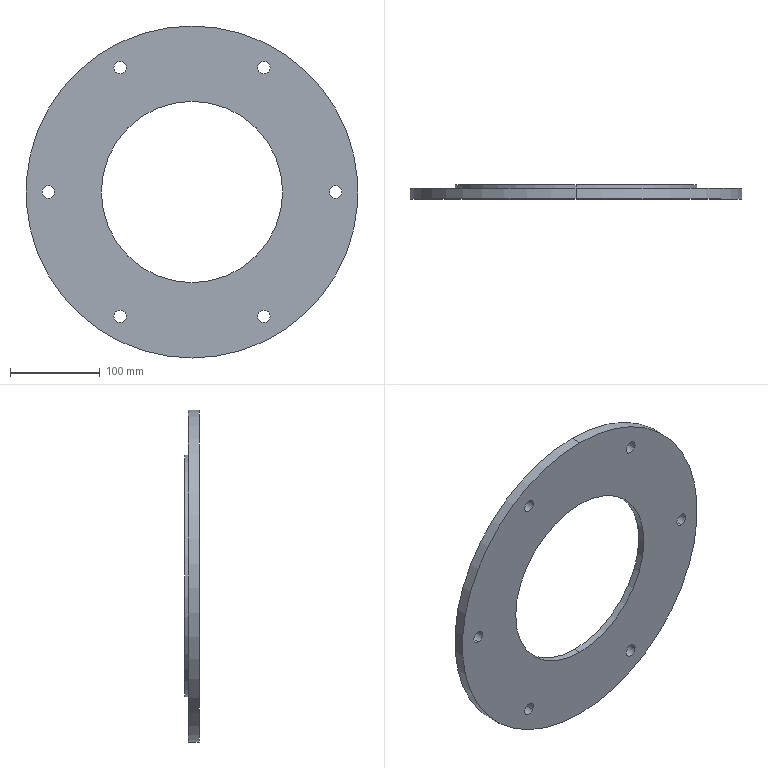Part | SolidWorks | features ICE 3, CirPattern 1, Extrusion 1 | 1 solid | 24 faces | box 370 x 16 x 370 mm | volume 827853 mm3 | cylinder 20 | plane 4 | commonest cylinder face diameters 14 x12 202 x2 259.5 x2 269.5 x2 370 x2
STEP:
#1=CARTESIAN_POINT('',(86.062,0.,135.064));
#2=VERTEX_POINT('',#1);
#3=CARTESIAN_POINT('',(73.938,0.,142.064));
#4=VERTEX_POINT('',#3);
#5=CARTESIAN_POINT('',(80.,0.,138.564));
#6=DIRECTION('',(0.,1.,0.));
#7=DIRECTION('',(-0.866,0.,0.5));
#8=AXIS2_PLACEMENT_3D('',#5,#6,#7);
#9=CIRCLE('',#8,7.);
#10=EDGE_CURVE('',#2,#4,#9,.T.);
#11=ORIENTED_EDGE('',*,*,#10,.F.);
#12=CARTESIAN_POINT('',(86.062,12.,135.064));
#13=VERTEX_POINT('',#12);
#14=CARTESIAN_POINT('',(86.062,0.,135.064));
#15=DIRECTION('',(0.,1.,0.));
#16=VECTOR('',#15,1000.);
#17=LINE('',#14,#16);
#18=EDGE_CURVE('',#2,#13,#17,.T.);
#19=ORIENTED_EDGE('',*,*,#18,.T.);
#20=CARTESIAN_POINT('',(73.938,12.,142.064));
#21=VERTEX_POINT('',#20);
#22=CARTESIAN_POINT('',(80.,12.,138.564));
#23=DIRECTION('',(0.,1.,0.));
#24=DIRECTION('',(-0.866,0.,0.5));
#25=AXIS2_PLACEMENT_3D('',#22,#23,#24);
#26=CIRCLE('',#25,7.);
#27=EDGE_CURVE('',#13,#21,#26,.T.);
#28=ORIENTED_EDGE('',*,*,#27,.T.);
#29=CARTESIAN_POINT('',(73.938,0.,142.064));
#30=DIRECTION('',(0.,1.,0.));
#31=VECTOR('',#30,1000.);
#32=LINE('',#29,#31);
#33=EDGE_CURVE('',#4,#21,#32,.T.);
#34=ORIENTED_EDGE('',*,*,#33,.F.);
#35=EDGE_LOOP('',(#11,#19,#28,#34));
#36=FACE_OUTER_BOUND('',#35,.T.);
#37=CARTESIAN_POINT('',(80.,0.,138.564));
#38=DIRECTION('',(0.,1.,0.));
#39=DIRECTION('',(-0.866,0.,0.5));
#40=AXIS2_PLACEMENT_3D('',#37,#38,#39);
#41=CYLINDRICAL_SURFACE('',#40,7.);
#42=ADVANCED_FACE('',(#36),#41,.F.);
#43=CARTESIAN_POINT('',(-73.938,0.,142.064));
#44=VERTEX_POINT('',#43);
#45=CARTESIAN_POINT('',(-86.062,0.,135.064));
#46=VERTEX_POINT('',#45);
#47=CARTESIAN_POINT('',(-80.,0.,138.564));
#48=DIRECTION('',(0.,1.,0.));
#49=DIRECTION('',(-0.866,0.,-0.5));
#50=AXIS2_PLACEMENT_3D('',#47,#48,#49);
#51=CIRCLE('',#50,7.);
#52=EDGE_CURVE('',#44,#46,#51,.T.);
#53=ORIENTED_EDGE('',*,*,#52,.F.);
#54=CARTESIAN_POINT('',(-73.938,12.,142.064));
#55=VERTEX_POINT('',#54);
#56=CARTESIAN_POINT('',(-73.938,0.,142.064));
#57=DIRECTION('',(0.,1.,0.));
#58=VECTOR('',#57,1000.);
#59=LINE('',#56,#58);
#60=EDGE_CURVE('',#44,#55,#59,.T.);
#61=ORIENTED_EDGE('',*,*,#60,.T.);
#62=CARTESIAN_POINT('',(-86.062,12.,135.064));
#63=VERTEX_POINT('',#62);
#64=CARTESIAN_POINT('',(-80.,12.,138.564));
#65=DIRECTION('',(0.,1.,0.));
#66=DIRECTION('',(-0.866,0.,-0.5));
#67=AXIS2_PLACEMENT_3D('',#64,#65,#66);
#68=CIRCLE('',#67,7.);
#69=EDGE_CURVE('',#55,#63,#68,.T.);
#70=ORIENTED_EDGE('',*,*,#69,.T.);
#71=CARTESIAN_POINT('',(-86.062,0.,135.064));
#72=DIRECTION('',(0.,1.,0.));
#73=VECTOR('',#72,1000.);
#74=LINE('',#71,#73);
#75=EDGE_CURVE('',#46,#63,#74,.T.);
#76=ORIENTED_EDGE('',*,*,#75,.F.);
#77=EDGE_LOOP('',(#53,#61,#70,#76));
#78=FACE_OUTER_BOUND('',#77,.T.);
#79=CARTESIAN_POINT('',(-80.,0.,138.564));
#80=DIRECTION('',(0.,1.,0.));
#81=DIRECTION('',(-0.866,0.,-0.5));
#82=AXIS2_PLACEMENT_3D('',#79,#80,#81);
#83=CYLINDRICAL_SURFACE('',#82,7.);
#84=ADVANCED_FACE('',(#78),#83,.F.);
#85=CARTESIAN_POINT('',(-160.,0.,7.));
#86=VERTEX_POINT('',#85);
#87=CARTESIAN_POINT('',(-160.,0.,-7.));
#88=VERTEX_POINT('',#87);
#89=CARTESIAN_POINT('',(-160.,0.,0.));
#90=DIRECTION('',(0.,1.,0.));
#91=DIRECTION('',(0.,0.,-1.));
#92=AXIS2_PLACEMENT_3D('',#89,#90,#91);
#93=CIRCLE('',#92,7.);
#94=EDGE_CURVE('',#86,#88,#93,.T.);
#95=ORIENTED_EDGE('',*,*,#94,.F.);
#96=CARTESIAN_POINT('',(-160.,12.,7.));
#97=VERTEX_POINT('',#96);
#98=CARTESIAN_POINT('',(-160.,0.,7.));
#99=DIRECTION('',(0.,1.,0.));
#100=VECTOR('',#99,1000.);
#101=LINE('',#98,#100);
#102=EDGE_CURVE('',#86,#97,#101,.T.);
#103=ORIENTED_EDGE('',*,*,#102,.T.);
#104=CARTESIAN_POINT('',(-160.,12.,-7.));
#105=VERTEX_POINT('',#104);
#106=CARTESIAN_POINT('',(-160.,12.,0.));
#107=DIRECTION('',(0.,1.,0.));
#108=DIRECTION('',(0.,0.,-1.));
#109=AXIS2_PLACEMENT_3D('',#106,#107,#108);
#110=CIRCLE('',#109,7.);
#111=EDGE_CURVE('',#97,#105,#110,.T.);
#112=ORIENTED_EDGE('',*,*,#111,.T.);
#113=CARTESIAN_POINT('',(-160.,0.,-7.));
#114=DIRECTION('',(0.,1.,0.));
#115=VECTOR('',#114,1000.);
#116=LINE('',#113,#115);
#117=EDGE_CURVE('',#88,#105,#116,.T.);
#118=ORIENTED_EDGE('',*,*,#117,.F.);
#119=EDGE_LOOP('',(#95,#103,#112,#118));
#120=FACE_OUTER_BOUND('',#119,.T.);
#121=CARTESIAN_POINT('',(-160.,0.,0.));
#122=DIRECTION('',(0.,1.,0.));
#123=DIRECTION('',(0.,0.,-1.));
#124=AXIS2_PLACEMENT_3D('',#121,#122,#123);
#125=CYLINDRICAL_SURFACE('',#124,7.);
#126=ADVANCED_FACE('',(#120),#125,.F.);
#127=CARTESIAN_POINT('',(-86.062,0.,-135.064));
#128=VERTEX_POINT('',#127);
#129=CARTESIAN_POINT('',(-73.938,0.,-142.064));
#130=VERTEX_POINT('',#129);
#131=CARTESIAN_POINT('',(-80.,0.,-138.564));
#132=DIRECTION('',(0.,1.,0.));
#133=DIRECTION('',(0.866,0.,-0.5));
#134=AXIS2_PLACEMENT_3D('',#131,#132,#133);
#135=CIRCLE('',#134,7.);
#136=EDGE_CURVE('',#128,#130,#135,.T.);
#137=ORIENTED_EDGE('',*,*,#136,.F.);
#138=CARTESIAN_POINT('',(-86.062,12.,-135.064));
#139=VERTEX_POINT('',#138);
#140=CARTESIAN_POINT('',(-86.062,0.,-135.064));
#141=DIRECTION('',(0.,1.,0.));
#142=VECTOR('',#141,1000.);
#143=LINE('',#140,#142);
#144=EDGE_CURVE('',#128,#139,#143,.T.);
#145=ORIENTED_EDGE('',*,*,#144,.T.);
#146=CARTESIAN_POINT('',(-73.938,12.,-142.064));
#147=VERTEX_POINT('',#146);
#148=CARTESIAN_POINT('',(-80.,12.,-138.564));
#149=DIRECTION('',(0.,1.,0.));
#150=DIRECTION('',(0.866,0.,-0.5));
#151=AXIS2_PLACEMENT_3D('',#148,#149,#150);
#152=CIRCLE('',#151,7.);
#153=EDGE_CURVE('',#139,#147,#152,.T.);
#154=ORIENTED_EDGE('',*,*,#153,.T.);
#155=CARTESIAN_POINT('',(-73.938,0.,-142.064));
#156=DIRECTION('',(0.,1.,0.));
#157=VECTOR('',#156,1000.);
#158=LINE('',#155,#157);
#159=EDGE_CURVE('',#130,#147,#158,.T.);
#160=ORIENTED_EDGE('',*,*,#159,.F.);
#161=EDGE_LOOP('',(#137,#145,#154,#160));
#162=FACE_OUTER_BOUND('',#161,.T.);
#163=CARTESIAN_POINT('',(-80.,0.,-138.564));
#164=DIRECTION('',(0.,1.,0.));
#165=DIRECTION('',(0.866,0.,-0.5));
#166=AXIS2_PLACEMENT_3D('',#163,#164,#165);
#167=CYLINDRICAL_SURFACE('',#166,7.);
#168=ADVANCED_FACE('',(#162),#167,.F.);
#169=CARTESIAN_POINT('',(73.938,0.,-142.064));
#170=VERTEX_POINT('',#169);
#171=CARTESIAN_POINT('',(86.062,0.,-135.064));
#172=VERTEX_POINT('',#171);
#173=CARTESIAN_POINT('',(80.,0.,-138.564));
#174=DIRECTION('',(0.,1.,0.));
#175=DIRECTION('',(0.866,0.,0.5));
#176=AXIS2_PLACEMENT_3D('',#173,#174,#175);
#177=CIRCLE('',#176,7.);
#178=EDGE_CURVE('',#170,#172,#177,.T.);
#179=ORIENTED_EDGE('',*,*,#178,.F.);
#180=CARTESIAN_POINT('',(73.938,12.,-142.064));
#181=VERTEX_POINT('',#180);
#182=CARTESIAN_POINT('',(73.938,0.,-142.064));
#183=DIRECTION('',(0.,1.,0.));
#184=VECTOR('',#183,1000.);
#185=LINE('',#182,#184);
#186=EDGE_CURVE('',#170,#181,#185,.T.);
#187=ORIENTED_EDGE('',*,*,#186,.T.);
#188=CARTESIAN_POINT('',(86.062,12.,-135.064));
#189=VERTEX_POINT('',#188);
#190=CARTESIAN_POINT('',(80.,12.,-138.564));
#191=DIRECTION('',(0.,1.,0.));
#192=DIRECTION('',(0.866,0.,0.5));
#193=AXIS2_PLACEMENT_3D('',#190,#191,#192);
#194=CIRCLE('',#193,7.);
#195=EDGE_CURVE('',#181,#189,#194,.T.);
#196=ORIENTED_EDGE('',*,*,#195,.T.);
#197=CARTESIAN_POINT('',(86.062,0.,-135.064));
#198=DIRECTION('',(0.,1.,0.));
#199=VECTOR('',#198,1000.);
#200=LINE('',#197,#199);
#201=EDGE_CURVE('',#172,#189,#200,.T.);
#202=ORIENTED_EDGE('',*,*,#201,.F.);
#203=EDGE_LOOP('',(#179,#187,#196,#202));
#204=FACE_OUTER_BOUND('',#203,.T.);
#205=CARTESIAN_POINT('',(80.,0.,-138.564));
#206=DIRECTION('',(0.,1.,0.));
#207=DIRECTION('',(0.866,0.,0.5));
#208=AXIS2_PLACEMENT_3D('',#205,#206,#207);
#209=CYLINDRICAL_SURFACE('',#208,7.);
#210=ADVANCED_FACE('',(#204),#209,.F.);
#211=CARTESIAN_POINT('',(160.,0.,-7.));
#212=VERTEX_POINT('',#211);
#213=CARTESIAN_POINT('',(160.,0.,7.));
#214=VERTEX_POINT('',#213);
#215=CARTESIAN_POINT('',(160.,0.,0.));
#216=DIRECTION('',(0.,1.,0.));
#217=DIRECTION('',(0.,0.,1.));
#218=AXIS2_PLACEMENT_3D('',#215,#216,#217);
#219=CIRCLE('',#218,7.);
#220=EDGE_CURVE('',#212,#214,#219,.T.);
#221=ORIENTED_EDGE('',*,*,#220,.F.);
#222=CARTESIAN_POINT('',(160.,12.,-7.));
#223=VERTEX_POINT('',#222);
#224=CARTESIAN_POINT('',(160.,0.,-7.));
#225=DIRECTION('',(0.,1.,0.));
#226=VECTOR('',#225,1000.);
#227=LINE('',#224,#226);
#228=EDGE_CURVE('',#212,#223,#227,.T.);
#229=ORIENTED_EDGE('',*,*,#228,.T.);
#230=CARTESIAN_POINT('',(160.,12.,7.));
#231=VERTEX_POINT('',#230);
#232=CARTESIAN_POINT('',(160.,12.,0.));
#233=DIRECTION('',(0.,1.,0.));
#234=DIRECTION('',(0.,0.,1.));
#235=AXIS2_PLACEMENT_3D('',#232,#233,#234);
#236=CIRCLE('',#235,7.);
#237=EDGE_CURVE('',#223,#231,#236,.T.);
#238=ORIENTED_EDGE('',*,*,#237,.T.);
#239=CARTESIAN_POINT('',(160.,0.,7.));
#240=DIRECTION('',(0.,1.,0.));
#241=VECTOR('',#240,1000.);
#242=LINE('',#239,#241);
#243=EDGE_CURVE('',#214,#231,#242,.T.);
#244=ORIENTED_EDGE('',*,*,#243,.F.);
#245=EDGE_LOOP('',(#221,#229,#238,#244));
#246=FACE_OUTER_BOUND('',#245,.T.);
#247=CARTESIAN_POINT('',(160.,0.,0.));
#248=DIRECTION('',(0.,1.,0.));
#249=DIRECTION('',(0.,0.,1.));
#250=AXIS2_PLACEMENT_3D('',#247,#248,#249);
#251=CYLINDRICAL_SURFACE('',#250,7.);
#252=ADVANCED_FACE('',(#246),#251,.F.);
#253=CARTESIAN_POINT('',(0.,16.,134.75));
#254=VERTEX_POINT('',#253);
#255=CARTESIAN_POINT('',(0.,16.,-134.75));
#256=VERTEX_POINT('',#255);
#257=CARTESIAN_POINT('',(0.,16.,0.));
#258=DIRECTION('',(0.,1.,0.));
#259=DIRECTION('',(0.,0.,1.));
#260=AXIS2_PLACEMENT_3D('',#257,#258,#259);
#261=CIRCLE('',#260,134.75);
#262=EDGE_CURVE('',#254,#256,#261,.T.);
#263=ORIENTED_EDGE('',*,*,#262,.F.);
#264=CARTESIAN_POINT('',(0.,12.,134.75));
#265=VERTEX_POINT('',#264);
#266=CARTESIAN_POINT('',(0.,16.,134.75));
#267=DIRECTION('',(0.,-1.,0.));
#268=VECTOR('',#267,1000.);
#269=LINE('',#266,#268);
#270=EDGE_CURVE('',#254,#265,#269,.T.);
#271=ORIENTED_EDGE('',*,*,#270,.T.);
#272=CARTESIAN_POINT('',(0.,12.,-134.75));
#273=VERTEX_POINT('',#272);
#274=CARTESIAN_POINT('',(0.,12.,0.));
#275=DIRECTION('',(0.,1.,0.));
#276=DIRECTION('',(0.,0.,1.));
#277=AXIS2_PLACEMENT_3D('',#274,#275,#276);
#278=CIRCLE('',#277,134.75);
#279=EDGE_CURVE('',#265,#273,#278,.T.);
#280=ORIENTED_EDGE('',*,*,#279,.T.);
#281=CARTESIAN_POINT('',(0.,16.,-134.75));
#282=DIRECTION('',(0.,-1.,0.));
#283=VECTOR('',#282,1000.);
#284=LINE('',#281,#283);
#285=EDGE_CURVE('',#256,#273,#284,.T.);
#286=ORIENTED_EDGE('',*,*,#285,.F.);
#287=EDGE_LOOP('',(#263,#271,#280,#286));
#288=FACE_OUTER_BOUND('',#287,.T.);
#289=CARTESIAN_POINT('',(0.,16.,0.));
#290=DIRECTION('',(0.,-1.,0.));
#291=DIRECTION('',(0.,0.,-1.));
#292=AXIS2_PLACEMENT_3D('',#289,#290,#291);
#293=CYLINDRICAL_SURFACE('',#292,134.75);
#294=ADVANCED_FACE('',(#288),#293,.T.);
#295=CARTESIAN_POINT('',(0.,8.,-129.75));
#296=VERTEX_POINT('',#295);
#297=CARTESIAN_POINT('',(0.,8.,129.75));
#298=VERTEX_POINT('',#297);
#299=CARTESIAN_POINT('',(0.,8.,0.));
#300=DIRECTION('',(0.,1.,0.));
#301=DIRECTION('',(0.,0.,1.));
#302=AXIS2_PLACEMENT_3D('',#299,#300,#301);
#303=CIRCLE('',#302,129.75);
#304=EDGE_CURVE('',#296,#298,#303,.T.);
#305=ORIENTED_EDGE('',*,*,#304,.F.);
#306=CARTESIAN_POINT('',(0.,16.,-129.75));
#307=VERTEX_POINT('',#306);
#308=CARTESIAN_POINT('',(0.,8.,-129.75));
#309=DIRECTION('',(0.,1.,0.));
#310=VECTOR('',#309,1000.);
#311=LINE('',#308,#310);
#312=EDGE_CURVE('',#296,#307,#311,.T.);
#313=ORIENTED_EDGE('',*,*,#312,.T.);
#314=CARTESIAN_POINT('',(0.,16.,129.75));
#315=VERTEX_POINT('',#314);
#316=CARTESIAN_POINT('',(0.,16.,0.));
#317=DIRECTION('',(0.,1.,0.));
#318=DIRECTION('',(0.,0.,1.));
#319=AXIS2_PLACEMENT_3D('',#316,#317,#318);
#320=CIRCLE('',#319,129.75);
#321=EDGE_CURVE('',#307,#315,#320,.T.);
#322=ORIENTED_EDGE('',*,*,#321,.T.);
#323=CARTESIAN_POINT('',(0.,8.,129.75));
#324=DIRECTION('',(0.,1.,0.));
#325=VECTOR('',#324,1000.);
#326=LINE('',#323,#325);
#327=EDGE_CURVE('',#298,#315,#326,.T.);
#328=ORIENTED_EDGE('',*,*,#327,.F.);
#329=EDGE_LOOP('',(#305,#313,#322,#328));
#330=FACE_OUTER_BOUND('',#329,.T.);
#331=CARTESIAN_POINT('',(0.,8.,0.));
#332=DIRECTION('',(0.,1.,0.));
#333=DIRECTION('',(0.,0.,1.));
#334=AXIS2_PLACEMENT_3D('',#331,#332,#333);
#335=CYLINDRICAL_SURFACE('',#334,129.75);
#336=ADVANCED_FACE('',(#330),#335,.F.);
#337=CARTESIAN_POINT('',(0.,12.,185.));
#338=VERTEX_POINT('',#337);
#339=CARTESIAN_POINT('',(0.,12.,-185.));
#340=VERTEX_POINT('',#339);
#341=CARTESIAN_POINT('',(0.,12.,0.));
#342=DIRECTION('',(0.,1.,0.));
#343=DIRECTION('',(0.,0.,1.));
#344=AXIS2_PLACEMENT_3D('',#341,#342,#343);
#345=CIRCLE('',#344,185.);
#346=EDGE_CURVE('',#338,#340,#345,.T.);
#347=ORIENTED_EDGE('',*,*,#346,.F.);
#348=CARTESIAN_POINT('',(0.,0.,185.));
#349=VERTEX_POINT('',#348);
#350=CARTESIAN_POINT('',(0.,12.,185.));
#351=DIRECTION('',(0.,-1.,0.));
#352=VECTOR('',#351,1000.);
#353=LINE('',#350,#352);
#354=EDGE_CURVE('',#338,#349,#353,.T.);
#355=ORIENTED_EDGE('',*,*,#354,.T.);
#356=CARTESIAN_POINT('',(0.,0.,-185.));
#357=VERTEX_POINT('',#356);
#358=CARTESIAN_POINT('',(0.,0.,0.));
#359=DIRECTION('',(0.,1.,0.));
#360=DIRECTION('',(0.,0.,1.));
#361=AXIS2_PLACEMENT_3D('',#358,#359,#360);
#362=CIRCLE('',#361,185.);
#363=EDGE_CURVE('',#349,#357,#362,.T.);
#364=ORIENTED_EDGE('',*,*,#363,.T.);
#365=CARTESIAN_POINT('',(0.,12.,-185.));
#366=DIRECTION('',(0.,-1.,0.));
#367=VECTOR('',#366,1000.);
#368=LINE('',#365,#367);
#369=EDGE_CURVE('',#340,#357,#368,.T.);
#370=ORIENTED_EDGE('',*,*,#369,.F.);
#371=EDGE_LOOP('',(#347,#355,#364,#370));
#372=FACE_OUTER_BOUND('',#371,.T.);
#373=CARTESIAN_POINT('',(0.,12.,0.));
#374=DIRECTION('',(0.,-1.,0.));
#375=DIRECTION('',(0.,0.,-1.));
#376=AXIS2_PLACEMENT_3D('',#373,#374,#375);
#377=CYLINDRICAL_SURFACE('',#376,185.);
#378=ADVANCED_FACE('',(#372),#377,.T.);
#379=CARTESIAN_POINT('',(0.,8.,-101.));
#380=VERTEX_POINT('',#379);
#381=CARTESIAN_POINT('',(0.,8.,101.));
#382=VERTEX_POINT('',#381);
#383=CARTESIAN_POINT('',(0.,8.,0.));
#384=DIRECTION('',(0.,1.,0.));
#385=DIRECTION('',(0.,0.,1.));
#386=AXIS2_PLACEMENT_3D('',#383,#384,#385);
#387=CIRCLE('',#386,101.);
#388=EDGE_CURVE('',#380,#382,#387,.T.);
#389=ORIENTED_EDGE('',*,*,#388,.T.);
#390=CARTESIAN_POINT('',(0.,0.,101.));
#391=VERTEX_POINT('',#390);
#392=CARTESIAN_POINT('',(0.,12.,101.));
#393=DIRECTION('',(0.,-1.,0.));
#394=VECTOR('',#393,1000.);
#395=LINE('',#392,#394);
#396=EDGE_CURVE('',#382,#391,#395,.T.);
#397=ORIENTED_EDGE('',*,*,#396,.T.);
#398=CARTESIAN_POINT('',(0.,0.,-101.));
#399=VERTEX_POINT('',#398);
#400=CARTESIAN_POINT('',(0.,0.,0.));
#401=DIRECTION('',(0.,1.,0.));
#402=DIRECTION('',(0.,0.,1.));
#403=AXIS2_PLACEMENT_3D('',#400,#401,#402);
#404=CIRCLE('',#403,101.);
#405=EDGE_CURVE('',#399,#391,#404,.T.);
#406=ORIENTED_EDGE('',*,*,#405,.F.);
#407=CARTESIAN_POINT('',(0.,12.,-101.));
#408=DIRECTION('',(0.,-1.,0.));
#409=VECTOR('',#408,1000.);
#410=LINE('',#407,#409);
#411=EDGE_CURVE('',#380,#399,#410,.T.);
#412=ORIENTED_EDGE('',*,*,#411,.F.);
#413=EDGE_LOOP('',(#389,#397,#406,#412));
#414=FACE_OUTER_BOUND('',#413,.T.);
#415=CARTESIAN_POINT('',(0.,12.,0.));
#416=DIRECTION('',(0.,-1.,0.));
#417=DIRECTION('',(0.,0.,-1.));
#418=AXIS2_PLACEMENT_3D('',#415,#416,#417);
#419=CYLINDRICAL_SURFACE('',#418,101.);
#420=ADVANCED_FACE('',(#414),#419,.F.);
#421=CARTESIAN_POINT('',(80.,12.,138.564));
#422=DIRECTION('',(0.,1.,0.));
#423=DIRECTION('',(-0.866,0.,0.5));
#424=AXIS2_PLACEMENT_3D('',#421,#422,#423);
#425=CIRCLE('',#424,7.);
#426=EDGE_CURVE('',#21,#13,#425,.T.);
#427=ORIENTED_EDGE('',*,*,#426,.F.);
#428=ORIENTED_EDGE('',*,*,#27,.F.);
#429=EDGE_LOOP('',(#427,#428));
#430=FACE_BOUND('',#429,.T.);
#431=CARTESIAN_POINT('',(-80.,12.,138.564));
#432=DIRECTION('',(0.,1.,0.));
#433=DIRECTION('',(-0.866,0.,-0.5));
#434=AXIS2_PLACEMENT_3D('',#431,#432,#433);
#435=CIRCLE('',#434,7.);
#436=EDGE_CURVE('',#63,#55,#435,.T.);
#437=ORIENTED_EDGE('',*,*,#436,.F.);
#438=ORIENTED_EDGE('',*,*,#69,.F.);
#439=EDGE_LOOP('',(#437,#438));
#440=FACE_BOUND('',#439,.T.);
#441=CARTESIAN_POINT('',(-160.,12.,0.));
#442=DIRECTION('',(0.,1.,0.));
#443=DIRECTION('',(0.,0.,-1.));
#444=AXIS2_PLACEMENT_3D('',#441,#442,#443);
#445=CIRCLE('',#444,7.);
#446=EDGE_CURVE('',#105,#97,#445,.T.);
#447=ORIENTED_EDGE('',*,*,#446,.F.);
#448=ORIENTED_EDGE('',*,*,#111,.F.);
#449=EDGE_LOOP('',(#447,#448));
#450=FACE_BOUND('',#449,.T.);
#451=CARTESIAN_POINT('',(-80.,12.,-138.564));
#452=DIRECTION('',(0.,1.,0.));
#453=DIRECTION('',(0.866,0.,-0.5));
#454=AXIS2_PLACEMENT_3D('',#451,#452,#453);
#455=CIRCLE('',#454,7.);
#456=EDGE_CURVE('',#147,#139,#455,.T.);
#457=ORIENTED_EDGE('',*,*,#456,.F.);
#458=ORIENTED_EDGE('',*,*,#153,.F.);
#459=EDGE_LOOP('',(#457,#458));
#460=FACE_BOUND('',#459,.T.);
#461=CARTESIAN_POINT('',(80.,12.,-138.564));
#462=DIRECTION('',(0.,1.,0.));
#463=DIRECTION('',(0.866,0.,0.5));
#464=AXIS2_PLACEMENT_3D('',#461,#462,#463);
#465=CIRCLE('',#464,7.);
#466=EDGE_CURVE('',#189,#181,#465,.T.);
#467=ORIENTED_EDGE('',*,*,#466,.F.);
#468=ORIENTED_EDGE('',*,*,#195,.F.);
#469=EDGE_LOOP('',(#467,#468));
#470=FACE_BOUND('',#469,.T.);
#471=CARTESIAN_POINT('',(160.,12.,0.));
#472=DIRECTION('',(0.,1.,0.));
#473=DIRECTION('',(0.,0.,1.));
#474=AXIS2_PLACEMENT_3D('',#471,#472,#473);
#475=CIRCLE('',#474,7.);
#476=EDGE_CURVE('',#231,#223,#475,.T.);
#477=ORIENTED_EDGE('',*,*,#476,.F.);
#478=ORIENTED_EDGE('',*,*,#237,.F.);
#479=EDGE_LOOP('',(#477,#478));
#480=FACE_BOUND('',#479,.T.);
#481=CARTESIAN_POINT('',(0.,12.,0.));
#482=DIRECTION('',(0.,1.,0.));
#483=DIRECTION('',(0.,0.,1.));
#484=AXIS2_PLACEMENT_3D('',#481,#482,#483);
#485=CIRCLE('',#484,185.);
#486=EDGE_CURVE('',#340,#338,#485,.T.);
#487=ORIENTED_EDGE('',*,*,#486,.T.);
#488=ORIENTED_EDGE('',*,*,#346,.T.);
#489=EDGE_LOOP('',(#487,#488));
#490=FACE_OUTER_BOUND('',#489,.T.);
#491=CARTESIAN_POINT('',(0.,12.,0.));
#492=DIRECTION('',(0.,1.,0.));
#493=DIRECTION('',(0.,0.,1.));
#494=AXIS2_PLACEMENT_3D('',#491,#492,#493);
#495=CIRCLE('',#494,134.75);
#496=EDGE_CURVE('',#273,#265,#495,.T.);
#497=ORIENTED_EDGE('',*,*,#496,.F.);
#498=ORIENTED_EDGE('',*,*,#279,.F.);
#499=EDGE_LOOP('',(#497,#498));
#500=FACE_BOUND('',#499,.T.);
#501=CARTESIAN_POINT('',(0.,12.,0.));
#502=DIRECTION('',(0.,1.,0.));
#503=DIRECTION('',(0.,0.,1.));
#504=AXIS2_PLACEMENT_3D('',#501,#502,#503);
#505=PLANE('',#504);
#506=ADVANCED_FACE('',(#430,#440,#450,#460,#470,#480,#490,#500),#505,.T.);
#507=ORIENTED_EDGE('',*,*,#396,.F.);
#508=CARTESIAN_POINT('',(0.,8.,0.));
#509=DIRECTION('',(0.,1.,0.));
#510=DIRECTION('',(0.,0.,1.));
#511=AXIS2_PLACEMENT_3D('',#508,#509,#510);
#512=CIRCLE('',#511,101.);
#513=EDGE_CURVE('',#382,#380,#512,.T.);
#514=ORIENTED_EDGE('',*,*,#513,.T.);
#515=ORIENTED_EDGE('',*,*,#411,.T.);
#516=CARTESIAN_POINT('',(0.,0.,0.));
#517=DIRECTION('',(0.,1.,0.));
#518=DIRECTION('',(0.,0.,1.));
#519=AXIS2_PLACEMENT_3D('',#516,#517,#518);
#520=CIRCLE('',#519,101.);
#521=EDGE_CURVE('',#391,#399,#520,.T.);
#522=ORIENTED_EDGE('',*,*,#521,.F.);
#523=EDGE_LOOP('',(#507,#514,#515,#522));
#524=FACE_OUTER_BOUND('',#523,.T.);
#525=CARTESIAN_POINT('',(0.,12.,0.));
#526=DIRECTION('',(0.,-1.,0.));
#527=DIRECTION('',(0.,0.,-1.));
#528=AXIS2_PLACEMENT_3D('',#525,#526,#527);
#529=CYLINDRICAL_SURFACE('',#528,101.);
#530=ADVANCED_FACE('',(#524),#529,.F.);
#531=CARTESIAN_POINT('',(80.,0.,138.564));
#532=DIRECTION('',(0.,1.,0.));
#533=DIRECTION('',(-0.866,0.,0.5));
#534=AXIS2_PLACEMENT_3D('',#531,#532,#533);
#535=CIRCLE('',#534,7.);
#536=EDGE_CURVE('',#4,#2,#535,.T.);
#537=ORIENTED_EDGE('',*,*,#536,.T.);
#538=ORIENTED_EDGE('',*,*,#10,.T.);
#539=EDGE_LOOP('',(#537,#538));
#540=FACE_BOUND('',#539,.T.);
#541=CARTESIAN_POINT('',(-80.,0.,138.564));
#542=DIRECTION('',(0.,1.,0.));
#543=DIRECTION('',(-0.866,0.,-0.5));
#544=AXIS2_PLACEMENT_3D('',#541,#542,#543);
#545=CIRCLE('',#544,7.);
#546=EDGE_CURVE('',#46,#44,#545,.T.);
#547=ORIENTED_EDGE('',*,*,#546,.T.);
#548=ORIENTED_EDGE('',*,*,#52,.T.);
#549=EDGE_LOOP('',(#547,#548));
#550=FACE_BOUND('',#549,.T.);
#551=CARTESIAN_POINT('',(-160.,0.,0.));
#552=DIRECTION('',(0.,1.,0.));
#553=DIRECTION('',(0.,0.,-1.));
#554=AXIS2_PLACEMENT_3D('',#551,#552,#553);
#555=CIRCLE('',#554,7.);
#556=EDGE_CURVE('',#88,#86,#555,.T.);
#557=ORIENTED_EDGE('',*,*,#556,.T.);
#558=ORIENTED_EDGE('',*,*,#94,.T.);
#559=EDGE_LOOP('',(#557,#558));
#560=FACE_BOUND('',#559,.T.);
#561=CARTESIAN_POINT('',(-80.,0.,-138.564));
#562=DIRECTION('',(0.,1.,0.));
#563=DIRECTION('',(0.866,0.,-0.5));
#564=AXIS2_PLACEMENT_3D('',#561,#562,#563);
#565=CIRCLE('',#564,7.);
#566=EDGE_CURVE('',#130,#128,#565,.T.);
#567=ORIENTED_EDGE('',*,*,#566,.T.);
#568=ORIENTED_EDGE('',*,*,#136,.T.);
#569=EDGE_LOOP('',(#567,#568));
#570=FACE_BOUND('',#569,.T.);
#571=CARTESIAN_POINT('',(80.,0.,-138.564));
#572=DIRECTION('',(0.,1.,0.));
#573=DIRECTION('',(0.866,0.,0.5));
#574=AXIS2_PLACEMENT_3D('',#571,#572,#573);
#575=CIRCLE('',#574,7.);
#576=EDGE_CURVE('',#172,#170,#575,.T.);
#577=ORIENTED_EDGE('',*,*,#576,.T.);
#578=ORIENTED_EDGE('',*,*,#178,.T.);
#579=EDGE_LOOP('',(#577,#578));
#580=FACE_BOUND('',#579,.T.);
#581=CARTESIAN_POINT('',(160.,0.,0.));
#582=DIRECTION('',(0.,1.,0.));
#583=DIRECTION('',(0.,0.,1.));
#584=AXIS2_PLACEMENT_3D('',#581,#582,#583);
#585=CIRCLE('',#584,7.);
#586=EDGE_CURVE('',#214,#212,#585,.T.);
#587=ORIENTED_EDGE('',*,*,#586,.T.);
#588=ORIENTED_EDGE('',*,*,#220,.T.);
#589=EDGE_LOOP('',(#587,#588));
#590=FACE_BOUND('',#589,.T.);
#591=CARTESIAN_POINT('',(0.,0.,0.));
#592=DIRECTION('',(0.,1.,0.));
#593=DIRECTION('',(0.,0.,1.));
#594=AXIS2_PLACEMENT_3D('',#591,#592,#593);
#595=CIRCLE('',#594,185.);
#596=EDGE_CURVE('',#357,#349,#595,.T.);
#597=ORIENTED_EDGE('',*,*,#596,.F.);
#598=ORIENTED_EDGE('',*,*,#363,.F.);
#599=EDGE_LOOP('',(#597,#598));
#600=FACE_OUTER_BOUND('',#599,.T.);
#601=ORIENTED_EDGE('',*,*,#405,.T.);
#602=ORIENTED_EDGE('',*,*,#521,.T.);
#603=EDGE_LOOP('',(#601,#602));
#604=FACE_BOUND('',#603,.T.);
#605=CARTESIAN_POINT('',(0.,0.,0.));
#606=DIRECTION('',(0.,1.,0.));
#607=DIRECTION('',(0.,0.,1.));
#608=AXIS2_PLACEMENT_3D('',#605,#606,#607);
#609=PLANE('',#608);
#610=ADVANCED_FACE('',(#540,#550,#560,#570,#580,#590,#600,#604),#609,.F.);
#611=ORIENTED_EDGE('',*,*,#354,.F.);
#612=ORIENTED_EDGE('',*,*,#486,.F.);
#613=ORIENTED_EDGE('',*,*,#369,.T.);
#614=ORIENTED_EDGE('',*,*,#596,.T.);
#615=EDGE_LOOP('',(#611,#612,#613,#614));
#616=FACE_OUTER_BOUND('',#615,.T.);
#617=CARTESIAN_POINT('',(0.,12.,0.));
#618=DIRECTION('',(0.,-1.,0.));
#619=DIRECTION('',(0.,0.,-1.));
#620=AXIS2_PLACEMENT_3D('',#617,#618,#619);
#621=CYLINDRICAL_SURFACE('',#620,185.);
#622=ADVANCED_FACE('',(#616),#621,.T.);
#623=ORIENTED_EDGE('',*,*,#312,.F.);
#624=CARTESIAN_POINT('',(0.,8.,0.));
#625=DIRECTION('',(0.,1.,0.));
#626=DIRECTION('',(0.,0.,1.));
#627=AXIS2_PLACEMENT_3D('',#624,#625,#626);
#628=CIRCLE('',#627,129.75);
#629=EDGE_CURVE('',#298,#296,#628,.T.);
#630=ORIENTED_EDGE('',*,*,#629,.F.);
#631=ORIENTED_EDGE('',*,*,#327,.T.);
#632=CARTESIAN_POINT('',(0.,16.,0.));
#633=DIRECTION('',(0.,1.,0.));
#634=DIRECTION('',(0.,0.,1.));
#635=AXIS2_PLACEMENT_3D('',#632,#633,#634);
#636=CIRCLE('',#635,129.75);
#637=EDGE_CURVE('',#315,#307,#636,.T.);
#638=ORIENTED_EDGE('',*,*,#637,.T.);
#639=EDGE_LOOP('',(#623,#630,#631,#638));
#640=FACE_OUTER_BOUND('',#639,.T.);
#641=CARTESIAN_POINT('',(0.,8.,0.));
#642=DIRECTION('',(0.,1.,0.));
#643=DIRECTION('',(0.,0.,1.));
#644=AXIS2_PLACEMENT_3D('',#641,#642,#643);
#645=CYLINDRICAL_SURFACE('',#644,129.75);
#646=ADVANCED_FACE('',(#640),#645,.F.);
#647=ORIENTED_EDGE('',*,*,#388,.F.);
#648=ORIENTED_EDGE('',*,*,#513,.F.);
#649=EDGE_LOOP('',(#647,#648));
#650=FACE_BOUND('',#649,.T.);
#651=ORIENTED_EDGE('',*,*,#629,.T.);
#652=ORIENTED_EDGE('',*,*,#304,.T.);
#653=EDGE_LOOP('',(#651,#652));
#654=FACE_OUTER_BOUND('',#653,.T.);
#655=CARTESIAN_POINT('',(0.,8.,0.));
#656=DIRECTION('',(0.,1.,0.));
#657=DIRECTION('',(0.,0.,1.));
#658=AXIS2_PLACEMENT_3D('',#655,#656,#657);
#659=PLANE('',#658);
#660=ADVANCED_FACE('',(#650,#654),#659,.T.);
#661=CARTESIAN_POINT('',(0.,16.,0.));
#662=DIRECTION('',(0.,1.,0.));
#663=DIRECTION('',(0.,0.,1.));
#664=AXIS2_PLACEMENT_3D('',#661,#662,#663);
#665=CIRCLE('',#664,134.75);
#666=EDGE_CURVE('',#256,#254,#665,.T.);
#667=ORIENTED_EDGE('',*,*,#666,.T.);
#668=ORIENTED_EDGE('',*,*,#262,.T.);
#669=EDGE_LOOP('',(#667,#668));
#670=FACE_OUTER_BOUND('',#669,.T.);
#671=ORIENTED_EDGE('',*,*,#637,.F.);
#672=ORIENTED_EDGE('',*,*,#321,.F.);
#673=EDGE_LOOP('',(#671,#672));
#674=FACE_BOUND('',#673,.T.);
#675=CARTESIAN_POINT('',(0.,16.,0.));
#676=DIRECTION('',(0.,1.,0.));
#677=DIRECTION('',(0.,0.,1.));
#678=AXIS2_PLACEMENT_3D('',#675,#676,#677);
#679=PLANE('',#678);
#680=ADVANCED_FACE('',(#670,#674),#679,.T.);
#681=ORIENTED_EDGE('',*,*,#270,.F.);
#682=ORIENTED_EDGE('',*,*,#666,.F.);
#683=ORIENTED_EDGE('',*,*,#285,.T.);
#684=ORIENTED_EDGE('',*,*,#496,.T.);
#685=EDGE_LOOP('',(#681,#682,#683,#684));
#686=FACE_OUTER_BOUND('',#685,.T.);
#687=CARTESIAN_POINT('',(0.,16.,0.));
#688=DIRECTION('',(0.,-1.,0.));
#689=DIRECTION('',(0.,0.,-1.));
#690=AXIS2_PLACEMENT_3D('',#687,#688,#689);
#691=CYLINDRICAL_SURFACE('',#690,134.75);
#692=ADVANCED_FACE('',(#686),#691,.T.);
#693=ORIENTED_EDGE('',*,*,#228,.F.);
#694=ORIENTED_EDGE('',*,*,#586,.F.);
#695=ORIENTED_EDGE('',*,*,#243,.T.);
#696=ORIENTED_EDGE('',*,*,#476,.T.);
#697=EDGE_LOOP('',(#693,#694,#695,#696));
#698=FACE_OUTER_BOUND('',#697,.T.);
#699=CARTESIAN_POINT('',(160.,0.,0.));
#700=DIRECTION('',(0.,1.,0.));
#701=DIRECTION('',(0.,0.,1.));
#702=AXIS2_PLACEMENT_3D('',#699,#700,#701);
#703=CYLINDRICAL_SURFACE('',#702,7.);
#704=ADVANCED_FACE('',(#698),#703,.F.);
#705=ORIENTED_EDGE('',*,*,#186,.F.);
#706=ORIENTED_EDGE('',*,*,#576,.F.);
#707=ORIENTED_EDGE('',*,*,#201,.T.);
#708=ORIENTED_EDGE('',*,*,#466,.T.);
#709=EDGE_LOOP('',(#705,#706,#707,#708));
#710=FACE_OUTER_BOUND('',#709,.T.);
#711=CARTESIAN_POINT('',(80.,0.,-138.564));
#712=DIRECTION('',(0.,1.,0.));
#713=DIRECTION('',(0.866,0.,0.5));
#714=AXIS2_PLACEMENT_3D('',#711,#712,#713);
#715=CYLINDRICAL_SURFACE('',#714,7.);
#716=ADVANCED_FACE('',(#710),#715,.F.);
#717=ORIENTED_EDGE('',*,*,#144,.F.);
#718=ORIENTED_EDGE('',*,*,#566,.F.);
#719=ORIENTED_EDGE('',*,*,#159,.T.);
#720=ORIENTED_EDGE('',*,*,#456,.T.);
#721=EDGE_LOOP('',(#717,#718,#719,#720));
#722=FACE_OUTER_BOUND('',#721,.T.);
#723=CARTESIAN_POINT('',(-80.,0.,-138.564));
#724=DIRECTION('',(0.,1.,0.));
#725=DIRECTION('',(0.866,0.,-0.5));
#726=AXIS2_PLACEMENT_3D('',#723,#724,#725);
#727=CYLINDRICAL_SURFACE('',#726,7.);
#728=ADVANCED_FACE('',(#722),#727,.F.);
#729=ORIENTED_EDGE('',*,*,#102,.F.);
#730=ORIENTED_EDGE('',*,*,#556,.F.);
#731=ORIENTED_EDGE('',*,*,#117,.T.);
#732=ORIENTED_EDGE('',*,*,#446,.T.);
#733=EDGE_LOOP('',(#729,#730,#731,#732));
#734=FACE_OUTER_BOUND('',#733,.T.);
#735=CARTESIAN_POINT('',(-160.,0.,0.));
#736=DIRECTION('',(0.,1.,0.));
#737=DIRECTION('',(0.,0.,-1.));
#738=AXIS2_PLACEMENT_3D('',#735,#736,#737);
#739=CYLINDRICAL_SURFACE('',#738,7.);
#740=ADVANCED_FACE('',(#734),#739,.F.);
#741=ORIENTED_EDGE('',*,*,#60,.F.);
#742=ORIENTED_EDGE('',*,*,#546,.F.);
#743=ORIENTED_EDGE('',*,*,#75,.T.);
#744=ORIENTED_EDGE('',*,*,#436,.T.);
#745=EDGE_LOOP('',(#741,#742,#743,#744));
#746=FACE_OUTER_BOUND('',#745,.T.);
#747=CARTESIAN_POINT('',(-80.,0.,138.564));
#748=DIRECTION('',(0.,1.,0.));
#749=DIRECTION('',(-0.866,0.,-0.5));
#750=AXIS2_PLACEMENT_3D('',#747,#748,#749);
#751=CYLINDRICAL_SURFACE('',#750,7.);
#752=ADVANCED_FACE('',(#746),#751,.F.);
#753=ORIENTED_EDGE('',*,*,#18,.F.);
#754=ORIENTED_EDGE('',*,*,#536,.F.);
#755=ORIENTED_EDGE('',*,*,#33,.T.);
#756=ORIENTED_EDGE('',*,*,#426,.T.);
#757=EDGE_LOOP('',(#753,#754,#755,#756));
#758=FACE_OUTER_BOUND('',#757,.T.);
#759=CARTESIAN_POINT('',(80.,0.,138.564));
#760=DIRECTION('',(0.,1.,0.));
#761=DIRECTION('',(-0.866,0.,0.5));
#762=AXIS2_PLACEMENT_3D('',#759,#760,#761);
#763=CYLINDRICAL_SURFACE('',#762,7.);
#764=ADVANCED_FACE('',(#758),#763,.F.);
#765=CLOSED_SHELL('',(#42,#84,#126,#168,#210,#252,#294,#336,#378,#420,#506,#530,#610,#622,#646,#660,#680,#692,#704,#716,#728,#740,#752,#764));
#766=MANIFOLD_SOLID_BREP('',#765);
#767=CARTESIAN_POINT('',(0.,0.,0.));
#768=DIRECTION('',(0.,0.,1.));
#769=DIRECTION('',(1.,0.,0.));
#770=AXIS2_PLACEMENT_3D('',#767,#768,#769);
#771=(LENGTH_UNIT()NAMED_UNIT(*)SI_UNIT(.MILLI.,.METRE.));
#772=UNCERTAINTY_MEASURE_WITH_UNIT(LENGTH_MEASURE(0.00001),#771,'','');
#773=(NAMED_UNIT(*)PLANE_ANGLE_UNIT()SI_UNIT($,.RADIAN.));
#774=(NAMED_UNIT(*)SI_UNIT($,.STERADIAN.)SOLID_ANGLE_UNIT());
#775=(GEOMETRIC_REPRESENTATION_CONTEXT(3)GLOBAL_UNCERTAINTY_ASSIGNED_CONTEXT((#772))GLOBAL_UNIT_ASSIGNED_CONTEXT((#771,#773,#774))REPRESENTATION_CONTEXT('',''));
#776=ADVANCED_BREP_SHAPE_REPRESENTATION('',(#766,#770),#775);